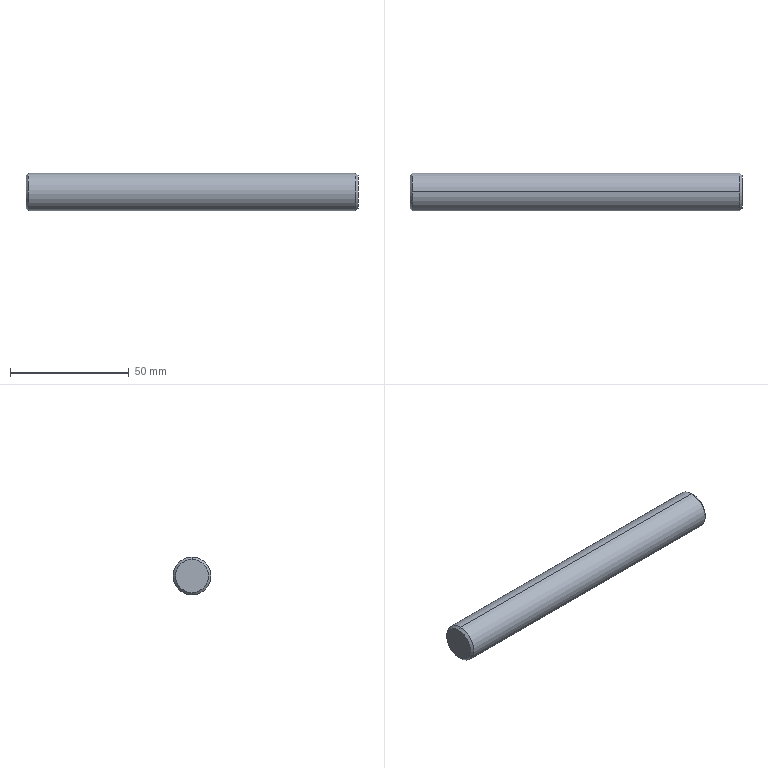Part | STEP file | BB67-M16-140L | 1 solid | 8 faces | box 140 x 16 x 16 mm | volume 28100 mm3 | cone 4 | cylinder 2 | plane 2 | commonest cylinder face diameters 16 x2
STEP:
#1=CARTESIAN_POINT('',(0.,0.,0.));
#2=DIRECTION('',(0.,0.,1.));
#3=DIRECTION('',(1.,0.,0.));
#4=AXIS2_PLACEMENT_3D('',#1,#2,#3);
#5=CARTESIAN_POINT('',(852.08,-824.04,659.327));
#6=VERTEX_POINT('',#5);
#7=CARTESIAN_POINT('',(852.08,-824.04,645.327));
#8=VERTEX_POINT('',#7);
#9=CARTESIAN_POINT('',(852.08,-824.04,652.327));
#10=DIRECTION('',(1.,0.,0.));
#11=DIRECTION('',(0.,0.,1.));
#12=AXIS2_PLACEMENT_3D('',#9,#10,#11);
#13=CIRCLE('',#12,7.);
#14=CARTESIAN_POINT('',(851.08,-824.04,652.327));
#15=DIRECTION('',(-1.,0.,0.));
#16=DIRECTION('',(0.,0.,-1.));
#17=AXIS2_PLACEMENT_3D('',#14,#15,#16);
#18=CONICAL_SURFACE('',#17,8.,0.7854);
#19=CARTESIAN_POINT('',(3.142,-1.));
#20=DIRECTION('',(-1.,0.));
#21=VECTOR('',#20,1.);
#22=LINE('',#19,#21);
#23=(GEOMETRIC_REPRESENTATION_CONTEXT(2)PARAMETRIC_REPRESENTATION_CONTEXT()REPRESENTATION_CONTEXT('',''));
#24=DEFINITIONAL_REPRESENTATION('',(#22),#23);
#25=PCURVE('',#18,#24);
#26=CARTESIAN_POINT('',(852.08,-824.04,652.327));
#27=DIRECTION('',(1.,0.,0.));
#28=DIRECTION('',(0.,0.,1.));
#29=AXIS2_PLACEMENT_3D('',#26,#27,#28);
#30=PLANE('',#29);
#31=CARTESIAN_POINT('',(0.,0.));
#32=DIRECTION('',(1.,0.));
#33=AXIS2_PLACEMENT_2D('',#31,#32);
#34=CIRCLE('',#33,7.);
#35=(GEOMETRIC_REPRESENTATION_CONTEXT(2)PARAMETRIC_REPRESENTATION_CONTEXT()REPRESENTATION_CONTEXT('',''));
#36=DEFINITIONAL_REPRESENTATION('',(#34),#35);
#37=PCURVE('',#30,#36);
#38=SURFACE_CURVE('',#13,(#25,#37),.PCURVE_S1.);
#39=EDGE_CURVE('',#6,#8,#38,.T.);
#40=ORIENTED_EDGE('',*,*,#39,.F.);
#41=CARTESIAN_POINT('',(851.08,-824.04,660.327));
#42=VERTEX_POINT('',#41);
#43=CARTESIAN_POINT('',(851.08,-824.04,660.327));
#44=DIRECTION('',(-0.7071,0.,0.7071));
#45=VECTOR('',#44,1.);
#46=LINE('',#43,#45);
#47=CARTESIAN_POINT('',(3.142,0.));
#48=DIRECTION('',(0.,1.));
#49=VECTOR('',#48,1.);
#50=LINE('',#47,#49);
#51=(GEOMETRIC_REPRESENTATION_CONTEXT(2)PARAMETRIC_REPRESENTATION_CONTEXT()REPRESENTATION_CONTEXT('',''));
#52=DEFINITIONAL_REPRESENTATION('',(#50),#51);
#53=PCURVE('',#18,#52);
#54=CARTESIAN_POINT('',(851.08,-824.04,652.327));
#55=DIRECTION('',(-1.,0.,0.));
#56=DIRECTION('',(0.,0.,-1.));
#57=AXIS2_PLACEMENT_3D('',#54,#55,#56);
#58=CONICAL_SURFACE('',#57,8.,0.7854);
#59=CARTESIAN_POINT('',(3.142,0.));
#60=DIRECTION('',(0.,1.));
#61=VECTOR('',#60,1.);
#62=LINE('',#59,#61);
#63=(GEOMETRIC_REPRESENTATION_CONTEXT(2)PARAMETRIC_REPRESENTATION_CONTEXT()REPRESENTATION_CONTEXT('',''));
#64=DEFINITIONAL_REPRESENTATION('',(#62),#63);
#65=PCURVE('',#58,#64);
#66=SURFACE_CURVE('',#46,(#53,#65),.PCURVE_S1.);
#67=EDGE_CURVE('',#6,#42,#66,.T.);
#68=ORIENTED_EDGE('',*,*,#67,.T.);
#69=CARTESIAN_POINT('',(851.08,-824.04,644.327));
#70=VERTEX_POINT('',#69);
#71=CARTESIAN_POINT('',(851.08,-824.04,652.327));
#72=DIRECTION('',(-1.,0.,0.));
#73=DIRECTION('',(0.,0.,1.));
#74=AXIS2_PLACEMENT_3D('',#71,#72,#73);
#75=CIRCLE('',#74,8.);
#76=CARTESIAN_POINT('',(-3.142,0.));
#77=DIRECTION('',(1.,0.));
#78=VECTOR('',#77,1.);
#79=LINE('',#76,#78);
#80=(GEOMETRIC_REPRESENTATION_CONTEXT(2)PARAMETRIC_REPRESENTATION_CONTEXT()REPRESENTATION_CONTEXT('',''));
#81=DEFINITIONAL_REPRESENTATION('',(#79),#80);
#82=PCURVE('',#18,#81);
#83=CARTESIAN_POINT('',(712.08,-824.04,652.327));
#84=DIRECTION('',(1.,0.,0.));
#85=DIRECTION('',(0.,0.,1.));
#86=AXIS2_PLACEMENT_3D('',#83,#84,#85);
#87=CYLINDRICAL_SURFACE('',#86,8.);
#88=CARTESIAN_POINT('',(6.283,139.));
#89=DIRECTION('',(-1.,0.));
#90=VECTOR('',#89,1.);
#91=LINE('',#88,#90);
#92=(GEOMETRIC_REPRESENTATION_CONTEXT(2)PARAMETRIC_REPRESENTATION_CONTEXT()REPRESENTATION_CONTEXT('',''));
#93=DEFINITIONAL_REPRESENTATION('',(#91),#92);
#94=PCURVE('',#87,#93);
#95=SURFACE_CURVE('',#75,(#82,#94),.PCURVE_S1.);
#96=EDGE_CURVE('',#70,#42,#95,.T.);
#97=ORIENTED_EDGE('',*,*,#96,.F.);
#98=CARTESIAN_POINT('',(851.08,-824.04,644.327));
#99=DIRECTION('',(-0.7071,0.,-0.7071));
#100=VECTOR('',#99,1.);
#101=LINE('',#98,#100);
#102=CARTESIAN_POINT('',(0.,0.));
#103=DIRECTION('',(0.,1.));
#104=VECTOR('',#103,1.);
#105=LINE('',#102,#104);
#106=(GEOMETRIC_REPRESENTATION_CONTEXT(2)PARAMETRIC_REPRESENTATION_CONTEXT()REPRESENTATION_CONTEXT('',''));
#107=DEFINITIONAL_REPRESENTATION('',(#105),#106);
#108=PCURVE('',#18,#107);
#109=CARTESIAN_POINT('',(6.283,0.));
#110=DIRECTION('',(0.,1.));
#111=VECTOR('',#110,1.);
#112=LINE('',#109,#111);
#113=(GEOMETRIC_REPRESENTATION_CONTEXT(2)PARAMETRIC_REPRESENTATION_CONTEXT()REPRESENTATION_CONTEXT('',''));
#114=DEFINITIONAL_REPRESENTATION('',(#112),#113);
#115=PCURVE('',#58,#114);
#116=SURFACE_CURVE('',#101,(#108,#115),.PCURVE_S1.);
#117=EDGE_CURVE('',#8,#70,#116,.T.);
#118=ORIENTED_EDGE('',*,*,#117,.F.);
#119=EDGE_LOOP('',(#40,#68,#97,#118));
#120=FACE_BOUND('',#119,.T.);
#121=ADVANCED_FACE('',(#120),#18,.T.);
#122=CARTESIAN_POINT('',(712.08,-824.04,645.327));
#123=VERTEX_POINT('',#122);
#124=CARTESIAN_POINT('',(712.08,-824.04,659.327));
#125=VERTEX_POINT('',#124);
#126=CARTESIAN_POINT('',(712.08,-824.04,652.327));
#127=DIRECTION('',(-1.,0.,0.));
#128=DIRECTION('',(0.,0.,-1.));
#129=AXIS2_PLACEMENT_3D('',#126,#127,#128);
#130=CIRCLE('',#129,7.);
#131=CARTESIAN_POINT('',(713.08,-824.04,652.327));
#132=DIRECTION('',(1.,0.,0.));
#133=DIRECTION('',(0.,0.,1.));
#134=AXIS2_PLACEMENT_3D('',#131,#132,#133);
#135=CONICAL_SURFACE('',#134,8.,0.7854);
#136=CARTESIAN_POINT('',(3.142,-1.));
#137=DIRECTION('',(-1.,0.));
#138=VECTOR('',#137,1.);
#139=LINE('',#136,#138);
#140=(GEOMETRIC_REPRESENTATION_CONTEXT(2)PARAMETRIC_REPRESENTATION_CONTEXT()REPRESENTATION_CONTEXT('',''));
#141=DEFINITIONAL_REPRESENTATION('',(#139),#140);
#142=PCURVE('',#135,#141);
#143=CARTESIAN_POINT('',(712.08,-824.04,652.327));
#144=DIRECTION('',(-1.,0.,0.));
#145=DIRECTION('',(0.,0.,-1.));
#146=AXIS2_PLACEMENT_3D('',#143,#144,#145);
#147=PLANE('',#146);
#148=CARTESIAN_POINT('',(0.,0.));
#149=DIRECTION('',(1.,0.));
#150=AXIS2_PLACEMENT_2D('',#148,#149);
#151=CIRCLE('',#150,7.);
#152=(GEOMETRIC_REPRESENTATION_CONTEXT(2)PARAMETRIC_REPRESENTATION_CONTEXT()REPRESENTATION_CONTEXT('',''));
#153=DEFINITIONAL_REPRESENTATION('',(#151),#152);
#154=PCURVE('',#147,#153);
#155=SURFACE_CURVE('',#130,(#142,#154),.PCURVE_S1.);
#156=EDGE_CURVE('',#123,#125,#155,.T.);
#157=ORIENTED_EDGE('',*,*,#156,.F.);
#158=CARTESIAN_POINT('',(713.08,-824.04,644.327));
#159=VERTEX_POINT('',#158);
#160=CARTESIAN_POINT('',(713.08,-824.04,644.327));
#161=DIRECTION('',(0.7071,0.,-0.7071));
#162=VECTOR('',#161,1.);
#163=LINE('',#160,#162);
#164=CARTESIAN_POINT('',(3.142,0.));
#165=DIRECTION('',(0.,1.));
#166=VECTOR('',#165,1.);
#167=LINE('',#164,#166);
#168=(GEOMETRIC_REPRESENTATION_CONTEXT(2)PARAMETRIC_REPRESENTATION_CONTEXT()REPRESENTATION_CONTEXT('',''));
#169=DEFINITIONAL_REPRESENTATION('',(#167),#168);
#170=PCURVE('',#135,#169);
#171=CARTESIAN_POINT('',(713.08,-824.04,652.327));
#172=DIRECTION('',(1.,0.,0.));
#173=DIRECTION('',(0.,0.,1.));
#174=AXIS2_PLACEMENT_3D('',#171,#172,#173);
#175=CONICAL_SURFACE('',#174,8.,0.7854);
#176=CARTESIAN_POINT('',(3.142,0.));
#177=DIRECTION('',(0.,1.));
#178=VECTOR('',#177,1.);
#179=LINE('',#176,#178);
#180=(GEOMETRIC_REPRESENTATION_CONTEXT(2)PARAMETRIC_REPRESENTATION_CONTEXT()REPRESENTATION_CONTEXT('',''));
#181=DEFINITIONAL_REPRESENTATION('',(#179),#180);
#182=PCURVE('',#175,#181);
#183=SURFACE_CURVE('',#163,(#170,#182),.PCURVE_S1.);
#184=EDGE_CURVE('',#123,#159,#183,.T.);
#185=ORIENTED_EDGE('',*,*,#184,.T.);
#186=CARTESIAN_POINT('',(713.08,-824.04,660.327));
#187=VERTEX_POINT('',#186);
#188=CARTESIAN_POINT('',(713.08,-824.04,652.327));
#189=DIRECTION('',(1.,0.,0.));
#190=DIRECTION('',(0.,0.,-1.));
#191=AXIS2_PLACEMENT_3D('',#188,#189,#190);
#192=CIRCLE('',#191,8.);
#193=CARTESIAN_POINT('',(-3.142,0.));
#194=DIRECTION('',(1.,0.));
#195=VECTOR('',#194,1.);
#196=LINE('',#193,#195);
#197=(GEOMETRIC_REPRESENTATION_CONTEXT(2)PARAMETRIC_REPRESENTATION_CONTEXT()REPRESENTATION_CONTEXT('',''));
#198=DEFINITIONAL_REPRESENTATION('',(#196),#197);
#199=PCURVE('',#135,#198);
#200=CARTESIAN_POINT('',(-3.142,1.));
#201=DIRECTION('',(1.,0.));
#202=VECTOR('',#201,1.);
#203=LINE('',#200,#202);
#204=(GEOMETRIC_REPRESENTATION_CONTEXT(2)PARAMETRIC_REPRESENTATION_CONTEXT()REPRESENTATION_CONTEXT('',''));
#205=DEFINITIONAL_REPRESENTATION('',(#203),#204);
#206=PCURVE('',#87,#205);
#207=SURFACE_CURVE('',#192,(#199,#206),.PCURVE_S1.);
#208=EDGE_CURVE('',#187,#159,#207,.T.);
#209=ORIENTED_EDGE('',*,*,#208,.F.);
#210=CARTESIAN_POINT('',(713.08,-824.04,660.327));
#211=DIRECTION('',(0.7071,0.,0.7071));
#212=VECTOR('',#211,1.);
#213=LINE('',#210,#212);
#214=CARTESIAN_POINT('',(0.,0.));
#215=DIRECTION('',(0.,1.));
#216=VECTOR('',#215,1.);
#217=LINE('',#214,#216);
#218=(GEOMETRIC_REPRESENTATION_CONTEXT(2)PARAMETRIC_REPRESENTATION_CONTEXT()REPRESENTATION_CONTEXT('',''));
#219=DEFINITIONAL_REPRESENTATION('',(#217),#218);
#220=PCURVE('',#135,#219);
#221=CARTESIAN_POINT('',(6.283,0.));
#222=DIRECTION('',(0.,1.));
#223=VECTOR('',#222,1.);
#224=LINE('',#221,#223);
#225=(GEOMETRIC_REPRESENTATION_CONTEXT(2)PARAMETRIC_REPRESENTATION_CONTEXT()REPRESENTATION_CONTEXT('',''));
#226=DEFINITIONAL_REPRESENTATION('',(#224),#225);
#227=PCURVE('',#175,#226);
#228=SURFACE_CURVE('',#213,(#220,#227),.PCURVE_S1.);
#229=EDGE_CURVE('',#125,#187,#228,.T.);
#230=ORIENTED_EDGE('',*,*,#229,.F.);
#231=EDGE_LOOP('',(#157,#185,#209,#230));
#232=FACE_BOUND('',#231,.T.);
#233=ADVANCED_FACE('',(#232),#135,.T.);
#234=ORIENTED_EDGE('',*,*,#208,.T.);
#235=CARTESIAN_POINT('',(712.08,-824.04,644.327));
#236=DIRECTION('',(1.,0.,0.));
#237=VECTOR('',#236,1.);
#238=LINE('',#235,#237);
#239=CARTESIAN_POINT('',(3.142,0.));
#240=DIRECTION('',(0.,1.));
#241=VECTOR('',#240,1.);
#242=LINE('',#239,#241);
#243=(GEOMETRIC_REPRESENTATION_CONTEXT(2)PARAMETRIC_REPRESENTATION_CONTEXT()REPRESENTATION_CONTEXT('',''));
#244=DEFINITIONAL_REPRESENTATION('',(#242),#243);
#245=PCURVE('',#87,#244);
#246=CARTESIAN_POINT('',(712.08,-824.04,652.327));
#247=DIRECTION('',(1.,0.,0.));
#248=DIRECTION('',(0.,0.,1.));
#249=AXIS2_PLACEMENT_3D('',#246,#247,#248);
#250=CYLINDRICAL_SURFACE('',#249,8.);
#251=CARTESIAN_POINT('',(3.142,0.));
#252=DIRECTION('',(0.,1.));
#253=VECTOR('',#252,1.);
#254=LINE('',#251,#253);
#255=(GEOMETRIC_REPRESENTATION_CONTEXT(2)PARAMETRIC_REPRESENTATION_CONTEXT()REPRESENTATION_CONTEXT('',''));
#256=DEFINITIONAL_REPRESENTATION('',(#254),#255);
#257=PCURVE('',#250,#256);
#258=SURFACE_CURVE('',#238,(#245,#257),.PCURVE_S1.);
#259=EDGE_CURVE('',#159,#70,#258,.T.);
#260=ORIENTED_EDGE('',*,*,#259,.T.);
#261=ORIENTED_EDGE('',*,*,#96,.T.);
#262=CARTESIAN_POINT('',(712.08,-824.04,660.327));
#263=DIRECTION('',(1.,0.,0.));
#264=VECTOR('',#263,1.);
#265=LINE('',#262,#264);
#266=CARTESIAN_POINT('',(0.,0.));
#267=DIRECTION('',(0.,1.));
#268=VECTOR('',#267,1.);
#269=LINE('',#266,#268);
#270=(GEOMETRIC_REPRESENTATION_CONTEXT(2)PARAMETRIC_REPRESENTATION_CONTEXT()REPRESENTATION_CONTEXT('',''));
#271=DEFINITIONAL_REPRESENTATION('',(#269),#270);
#272=PCURVE('',#87,#271);
#273=CARTESIAN_POINT('',(6.283,0.));
#274=DIRECTION('',(0.,1.));
#275=VECTOR('',#274,1.);
#276=LINE('',#273,#275);
#277=(GEOMETRIC_REPRESENTATION_CONTEXT(2)PARAMETRIC_REPRESENTATION_CONTEXT()REPRESENTATION_CONTEXT('',''));
#278=DEFINITIONAL_REPRESENTATION('',(#276),#277);
#279=PCURVE('',#250,#278);
#280=SURFACE_CURVE('',#265,(#272,#279),.PCURVE_S1.);
#281=EDGE_CURVE('',#187,#42,#280,.T.);
#282=ORIENTED_EDGE('',*,*,#281,.F.);
#283=EDGE_LOOP('',(#234,#260,#261,#282));
#284=FACE_BOUND('',#283,.T.);
#285=ADVANCED_FACE('',(#284),#87,.T.);
#286=CARTESIAN_POINT('',(852.08,-824.04,652.327));
#287=DIRECTION('',(1.,0.,0.));
#288=DIRECTION('',(0.,0.,1.));
#289=AXIS2_PLACEMENT_3D('',#286,#287,#288);
#290=CIRCLE('',#289,7.);
#291=CARTESIAN_POINT('',(0.,0.));
#292=DIRECTION('',(1.,0.));
#293=AXIS2_PLACEMENT_2D('',#291,#292);
#294=CIRCLE('',#293,7.);
#295=(GEOMETRIC_REPRESENTATION_CONTEXT(2)PARAMETRIC_REPRESENTATION_CONTEXT()REPRESENTATION_CONTEXT('',''));
#296=DEFINITIONAL_REPRESENTATION('',(#294),#295);
#297=PCURVE('',#30,#296);
#298=CARTESIAN_POINT('',(9.425,-1.));
#299=DIRECTION('',(-1.,0.));
#300=VECTOR('',#299,1.);
#301=LINE('',#298,#300);
#302=(GEOMETRIC_REPRESENTATION_CONTEXT(2)PARAMETRIC_REPRESENTATION_CONTEXT()REPRESENTATION_CONTEXT('',''));
#303=DEFINITIONAL_REPRESENTATION('',(#301),#302);
#304=PCURVE('',#58,#303);
#305=SURFACE_CURVE('',#290,(#297,#304),.PCURVE_S1.);
#306=EDGE_CURVE('',#8,#6,#305,.T.);
#307=ORIENTED_EDGE('',*,*,#306,.T.);
#308=ORIENTED_EDGE('',*,*,#39,.T.);
#309=EDGE_LOOP('',(#307,#308));
#310=FACE_BOUND('',#309,.T.);
#311=ADVANCED_FACE('',(#310),#30,.T.);
#312=CARTESIAN_POINT('',(712.08,-824.04,652.327));
#313=DIRECTION('',(-1.,0.,0.));
#314=DIRECTION('',(0.,0.,-1.));
#315=AXIS2_PLACEMENT_3D('',#312,#313,#314);
#316=CIRCLE('',#315,7.);
#317=CARTESIAN_POINT('',(0.,0.));
#318=DIRECTION('',(1.,0.));
#319=AXIS2_PLACEMENT_2D('',#317,#318);
#320=CIRCLE('',#319,7.);
#321=(GEOMETRIC_REPRESENTATION_CONTEXT(2)PARAMETRIC_REPRESENTATION_CONTEXT()REPRESENTATION_CONTEXT('',''));
#322=DEFINITIONAL_REPRESENTATION('',(#320),#321);
#323=PCURVE('',#147,#322);
#324=CARTESIAN_POINT('',(9.425,-1.));
#325=DIRECTION('',(-1.,0.));
#326=VECTOR('',#325,1.);
#327=LINE('',#324,#326);
#328=(GEOMETRIC_REPRESENTATION_CONTEXT(2)PARAMETRIC_REPRESENTATION_CONTEXT()REPRESENTATION_CONTEXT('',''));
#329=DEFINITIONAL_REPRESENTATION('',(#327),#328);
#330=PCURVE('',#175,#329);
#331=SURFACE_CURVE('',#316,(#323,#330),.PCURVE_S1.);
#332=EDGE_CURVE('',#125,#123,#331,.T.);
#333=ORIENTED_EDGE('',*,*,#332,.T.);
#334=ORIENTED_EDGE('',*,*,#156,.T.);
#335=EDGE_LOOP('',(#333,#334));
#336=FACE_BOUND('',#335,.T.);
#337=ADVANCED_FACE('',(#336),#147,.T.);
#338=ORIENTED_EDGE('',*,*,#259,.F.);
#339=CARTESIAN_POINT('',(713.08,-824.04,652.327));
#340=DIRECTION('',(1.,0.,0.));
#341=DIRECTION('',(0.,0.,-1.));
#342=AXIS2_PLACEMENT_3D('',#339,#340,#341);
#343=CIRCLE('',#342,8.);
#344=CARTESIAN_POINT('',(3.142,1.));
#345=DIRECTION('',(1.,0.));
#346=VECTOR('',#345,1.);
#347=LINE('',#344,#346);
#348=(GEOMETRIC_REPRESENTATION_CONTEXT(2)PARAMETRIC_REPRESENTATION_CONTEXT()REPRESENTATION_CONTEXT('',''));
#349=DEFINITIONAL_REPRESENTATION('',(#347),#348);
#350=PCURVE('',#250,#349);
#351=CARTESIAN_POINT('',(3.142,0.));
#352=DIRECTION('',(1.,0.));
#353=VECTOR('',#352,1.);
#354=LINE('',#351,#353);
#355=(GEOMETRIC_REPRESENTATION_CONTEXT(2)PARAMETRIC_REPRESENTATION_CONTEXT()REPRESENTATION_CONTEXT('',''));
#356=DEFINITIONAL_REPRESENTATION('',(#354),#355);
#357=PCURVE('',#175,#356);
#358=SURFACE_CURVE('',#343,(#350,#357),.PCURVE_S1.);
#359=EDGE_CURVE('',#159,#187,#358,.T.);
#360=ORIENTED_EDGE('',*,*,#359,.T.);
#361=ORIENTED_EDGE('',*,*,#281,.T.);
#362=CARTESIAN_POINT('',(851.08,-824.04,652.327));
#363=DIRECTION('',(-1.,0.,0.));
#364=DIRECTION('',(0.,0.,1.));
#365=AXIS2_PLACEMENT_3D('',#362,#363,#364);
#366=CIRCLE('',#365,8.);
#367=CARTESIAN_POINT('',(6.283,139.));
#368=DIRECTION('',(-1.,0.));
#369=VECTOR('',#368,1.);
#370=LINE('',#367,#369);
#371=(GEOMETRIC_REPRESENTATION_CONTEXT(2)PARAMETRIC_REPRESENTATION_CONTEXT()REPRESENTATION_CONTEXT('',''));
#372=DEFINITIONAL_REPRESENTATION('',(#370),#371);
#373=PCURVE('',#250,#372);
#374=CARTESIAN_POINT('',(3.142,0.));
#375=DIRECTION('',(1.,0.));
#376=VECTOR('',#375,1.);
#377=LINE('',#374,#376);
#378=(GEOMETRIC_REPRESENTATION_CONTEXT(2)PARAMETRIC_REPRESENTATION_CONTEXT()REPRESENTATION_CONTEXT('',''));
#379=DEFINITIONAL_REPRESENTATION('',(#377),#378);
#380=PCURVE('',#58,#379);
#381=SURFACE_CURVE('',#366,(#373,#380),.PCURVE_S1.);
#382=EDGE_CURVE('',#42,#70,#381,.T.);
#383=ORIENTED_EDGE('',*,*,#382,.T.);
#384=EDGE_LOOP('',(#338,#360,#361,#383));
#385=FACE_BOUND('',#384,.T.);
#386=ADVANCED_FACE('',(#385),#250,.T.);
#387=ORIENTED_EDGE('',*,*,#184,.F.);
#388=ORIENTED_EDGE('',*,*,#332,.F.);
#389=ORIENTED_EDGE('',*,*,#229,.T.);
#390=ORIENTED_EDGE('',*,*,#359,.F.);
#391=EDGE_LOOP('',(#387,#388,#389,#390));
#392=FACE_BOUND('',#391,.T.);
#393=ADVANCED_FACE('',(#392),#175,.T.);
#394=ORIENTED_EDGE('',*,*,#67,.F.);
#395=ORIENTED_EDGE('',*,*,#306,.F.);
#396=ORIENTED_EDGE('',*,*,#117,.T.);
#397=ORIENTED_EDGE('',*,*,#382,.F.);
#398=EDGE_LOOP('',(#394,#395,#396,#397));
#399=FACE_BOUND('',#398,.T.);
#400=ADVANCED_FACE('',(#399),#58,.T.);
#401=CLOSED_SHELL('',(#121,#233,#285,#311,#337,#386,#393,#400));
#402=MANIFOLD_SOLID_BREP('',#401);
#403=(LENGTH_UNIT()NAMED_UNIT(*)SI_UNIT(.MILLI.,.METRE.));
#404=UNCERTAINTY_MEASURE_WITH_UNIT(LENGTH_MEASURE(0.0000001),#403,'','');
#405=(NAMED_UNIT(*)PLANE_ANGLE_UNIT()SI_UNIT($,.RADIAN.));
#406=(NAMED_UNIT(*)SI_UNIT($,.STERADIAN.)SOLID_ANGLE_UNIT());
#407=(GEOMETRIC_REPRESENTATION_CONTEXT(3)GLOBAL_UNCERTAINTY_ASSIGNED_CONTEXT((#404))GLOBAL_UNIT_ASSIGNED_CONTEXT((#403,#405,#406))REPRESENTATION_CONTEXT('',''));
#408=ADVANCED_BREP_SHAPE_REPRESENTATION('',(#4,#402),#407);